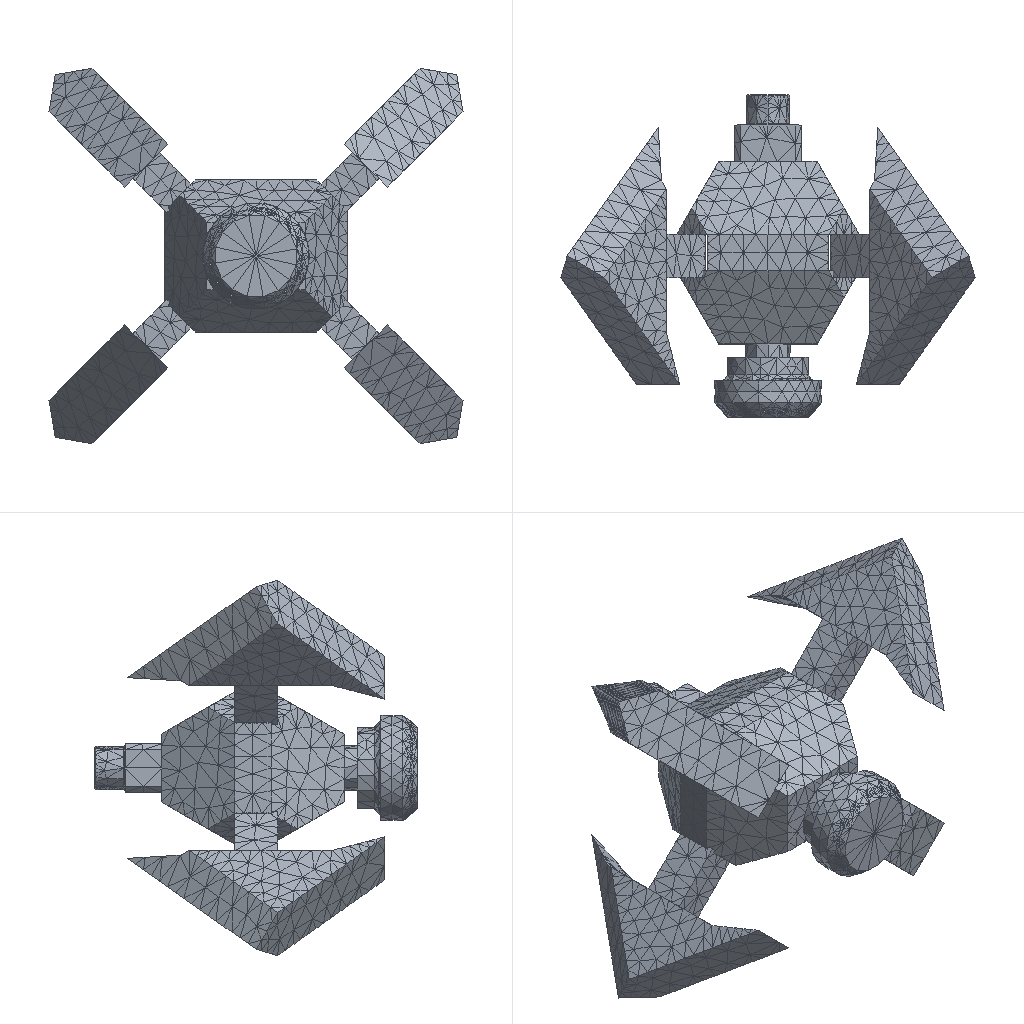Simulation study | ansys workbench
Set-up summary:
category,name,step,type,value,unit,region
solver,ansys_workbench
units,mm-N-s-tonne (MPa),,stated,"/units,MPA"
analysis,LS1,,static
load_step,LS1,LS1,static,nsubst=1; time=1
mesh,nodes,,,44105
mesh,elements,,,24845
element_type,SOLID187,,,22843
element_type,TARGE170,,,815
element_type,CONTA174,,,815
element_type,SURF154,,,230
element_type,SOLID186,,,142
material,Structural Steel,,E,200000,tonne s^-2 mm^-1
material,Structural Steel,,nu,0.3
material,Structural Steel,,density,7.85e-09,tonne mm^-3
material,Structural Steel,,conductivity,60.5,tonne mm s^-3 C^-1
material,Structural Steel,,specific_heat,4.34e+08,mm^2 s^-2 C^-1
material,Structural Steel,,cte,1.2e-05,C^-1
material,Structural Steel,,permeability,10000
material,Structural Steel,,resistivity,0.00017,ohm mm
load,"Define Pressure Using Surface Effect Elements ""__""",LS1,pressure,0.05,,SURF154 #25
load,Define Force Using Surface Effect Elements,LS1,surface-effect pres face 2,-0.01863,,SURF154 #26
bc,Fixed Supports,model,fixed,[dofs=ALL],,_FIXEDSU
contact,Contact Region,,bonded (always),element=CONTA174
contact,Contact Region 2,,bonded (always),element=CONTA174
contact,Contact Region 3,,bonded (always),element=CONTA174
contact,Contact Region 4,,bonded (always),element=CONTA174
contact,Contact Region 5,,bonded (always),element=CONTA174
contact,Contact Region 6,,bonded (always),element=CONTA174
contact,Contact Region 7,,bonded (always),element=CONTA174
contact,Contact Region 8,,bonded (always),element=CONTA174
named_set,_FIXEDSU,,node,980
Ansys APDL input file, long lists of numbers shortened:
/batch
/config,noeldb,1     ! force off writing results to database
*get,_wallstrt,active,,time,wall
! ANSYS input file written by Workbench version 2022 R1
! File used for geometry attach:
/title,wbnew--____ (B5)
! ****** Begin Custom Load Command Snippet ******
/COM, ACT Extensions:
/COM,     LSDYNA, 2021.1
/COM,
! ****** End   Custom Load Command Snippet ******
*DIM,_wb_ProjectScratch_dir,string,248
_wb_ProjectScratch_dir(1) = ''
*DIM,_wb_SolverFiles_dir,string,248
_wb_SolverFiles_dir(1) = ''
*DIM,_wb_userfiles_dir,string,248
_wb_userfiles_dir(1) = ''
/com,--- Data in consistent NMM units. See Solving Units in the help system for more information.
/units,MPA
/nopr
/wb,file,start              !  signify a WB generated input file
/prep7
! Turn off shape checking because checks already performed inside WB mesher.
! See help system for more information.
SHPP,OFF,,NOWARN
/nolist
etcon,set             ! allow ANSYS to choose best KEYOP's for 180x elements, resets any applicable keyopt to MAPDL defaults
/com,*********** Nodes for the whole assembly ***********
nblock,3,,48515
(1i9,3e20.9e3)
        1     5.028046008E+01     2.042995881E+02    -1.157319943E+01
! (44104 more lines like these left out)
-1
/wb,elem,start            !  set before creation of elements
/com,*********** Elements for Body 1 "__|__1" ***********
et,1,187
eblock,19,solid,,1525
(19i9)
        1        1        1        1        0        0        0        0       10        0      143     1288     1380     1470     1477     2782     3319     2784     2785
! (3049 more lines like these left out)
-1
/com,*********** Elements for Body 2 "___|___1" ***********
et,2,187
eblock,19,solid,,9956
(19i9)
        2        2        2        2        0        0        0        0       10        0    13030    29622    30030    29741    29839    43103    43625    43098    43100
! (19911 more lines like these left out)
-1
/com,*********** Elements for Body 3 "____|__-__1" ***********
et,3,186
keyo,3,2,1          ! set full integration on SOLID186
eblock,19,solid,,142
(19i9)
        3        3        3        3        0        0        0        0       20        0        1        7      316       13      153       26      315       20      163
! (283 more lines like these left out)
-1
/com,*********** Elements for Body 4 "___|__2" ***********
et,4,187
eblock,19,solid,,3028
(19i9)
        4        4        4        4        0        0        0        0       10        0     6243    13936    13937    14647    14646    17128    17151    17141    17140
! (6055 more lines like these left out)
-1
/com,*********** Elements for Body 5 "__|__1" ***********
et,5,187
eblock,19,solid,,3759
(19i9)
        5        5        5        5        0        0        0        0       10        0     9271    20224    21134    20732    21129    24359    26317    24356    24358
! (7517 more lines like these left out)
-1
/com,*********** Elements for Body 6 "__|__1[2]" ***********
et,6,187
eblock,19,solid,,1525
(19i9)
        6        6        6        6        0        0        0        0       10        0     4718    10588    10680    10770    10777    12082    12619    12084    12085
! (3049 more lines like these left out)
-1
/com,*********** Elements for Body 7 "__|__1[3]" ***********
et,7,187
eblock,19,solid,,1525
(19i9)
        7        7        7        7        0        0        0        0       10        0     1668     4388     4480     4570     4577     5882     6419     5884     5885
! (3049 more lines like these left out)
-1
/com,*********** Elements for Body 8 "__|__1[4]" ***********
et,8,187
eblock,19,solid,,1525
(19i9)
        8        8        8        8        0        0        0        0       10        0     3193     7488     7580     7670     7677     8982     9519     8984     8985
! (3049 more lines like these left out)
-1
/wb,elem,end               !  done creating elements
/com,*********** Send User Defined Coordinate System(s) ***********
csys,0
toffst,273.15,  ! Temperature offset from absolute zero
/com,*********** Set Reference Temperature ***********
tref,22.
/wb,mat,start              !  starting to send materials
/com,*********** Send Materials ***********
Temperature = 'TEMP' ! Temperature
MP,DENS,1,7.85e-09,	! tonne mm^-3
MP,ALPX,1,1.2e-05,	! C^-1
MP,C,1,434000000,	! mm^2 s^-2 C^-1
MP,KXX,1,60.5,	! tonne mm s^-3 C^-1
MP,RSVX,1,0.00017,	! ohm mm
MP,EX,1,200000,	! tonne s^-2 mm^-1
MP,NUXY,1,0.3,
MP,MURX,1,10000,
Temperature = 'TEMP' ! Temperature
MP,DENS,2,7.85e-09,	! tonne mm^-3
MP,ALPX,2,1.2e-05,	! C^-1
MP,C,2,434000000,	! mm^2 s^-2 C^-1
MP,KXX,2,60.5,	! tonne mm s^-3 C^-1
MP,RSVX,2,0.00017,	! ohm mm
MP,EX,2,200000,	! tonne s^-2 mm^-1
MP,NUXY,2,0.3,
MP,MURX,2,10000,
Temperature = 'TEMP' ! Temperature
MP,DENS,3,7.85e-09,	! tonne mm^-3
MP,ALPX,3,1.2e-05,	! C^-1
MP,C,3,434000000,	! mm^2 s^-2 C^-1
MP,KXX,3,60.5,	! tonne mm s^-3 C^-1
MP,RSVX,3,0.00017,	! ohm mm
MP,EX,3,200000,	! tonne s^-2 mm^-1
MP,NUXY,3,0.3,
MP,MURX,3,10000,
Temperature = 'TEMP' ! Temperature
MP,DENS,4,7.85e-09,	! tonne mm^-3
MP,ALPX,4,1.2e-05,	! C^-1
MP,C,4,434000000,	! mm^2 s^-2 C^-1
MP,KXX,4,60.5,	! tonne mm s^-3 C^-1
MP,RSVX,4,0.00017,	! ohm mm
MP,EX,4,200000,	! tonne s^-2 mm^-1
MP,NUXY,4,0.3,
MP,MURX,4,10000,
Temperature = 'TEMP' ! Temperature
MP,DENS,5,7.85e-09,	! tonne mm^-3
MP,ALPX,5,1.2e-05,	! C^-1
MP,C,5,434000000,	! mm^2 s^-2 C^-1
MP,KXX,5,60.5,	! tonne mm s^-3 C^-1
MP,RSVX,5,0.00017,	! ohm mm
MP,EX,5,200000,	! tonne s^-2 mm^-1
MP,NUXY,5,0.3,
MP,MURX,5,10000,
Temperature = 'TEMP' ! Temperature
MP,DENS,6,7.85e-09,	! tonne mm^-3
MP,ALPX,6,1.2e-05,	! C^-1
MP,C,6,434000000,	! mm^2 s^-2 C^-1
MP,KXX,6,60.5,	! tonne mm s^-3 C^-1
MP,RSVX,6,0.00017,	! ohm mm
MP,EX,6,200000,	! tonne s^-2 mm^-1
MP,NUXY,6,0.3,
MP,MURX,6,10000,
Temperature = 'TEMP' ! Temperature
MP,DENS,7,7.85e-09,	! tonne mm^-3
MP,ALPX,7,1.2e-05,	! C^-1
MP,C,7,434000000,	! mm^2 s^-2 C^-1
MP,KXX,7,60.5,	! tonne mm s^-3 C^-1
MP,RSVX,7,0.00017,	! ohm mm
MP,EX,7,200000,	! tonne s^-2 mm^-1
MP,NUXY,7,0.3,
MP,MURX,7,10000,
Temperature = 'TEMP' ! Temperature
MP,DENS,8,7.85e-09,	! tonne mm^-3
MP,ALPX,8,1.2e-05,	! C^-1
MP,C,8,434000000,	! mm^2 s^-2 C^-1
MP,KXX,8,60.5,	! tonne mm s^-3 C^-1
MP,RSVX,8,0.00017,	! ohm mm
MP,EX,8,200000,	! tonne s^-2 mm^-1
MP,NUXY,8,0.3,
MP,MURX,8,10000,
/wb,mat,end                !  done sending materials
!************************* Model Summary ********************
!__|__1,	结构钢,	matid,	1
!___|___1,	结构钢,	matid,	2
!____|__-__1,	结构钢,	matid,	3
!___|__2,	结构钢,	matid,	4
!__|__1,	结构钢,	matid,	5
!__|__1[2],	结构钢,	matid,	6
!__|__1[3],	结构钢,	matid,	7
!__|__1[4],	结构钢,	matid,	8
!************************* End Model Summary ********************
! get the diagonal of the bounding box. Needed later for other things
*get,_xmin,node,,mnloc,x
*get,_ymin,node,,mnloc,y
*get,_zmin,node,,mnloc,z
*get,_xmax,node,,mxloc,x
*get,_ymax,node,,mxloc,y
*get,_zmax,node,,mxloc,z
_ASMDIAG=(_xmax-_xmin)*(_xmax-_xmin)+(_ymax-_ymin)*(_ymax-_ymin)+(_zmax-_zmin)*(_zmax-_zmin)
_ASMDIAG=SQRT(_ASMDIAG)
/wb,contact,start          !  starting to send contact
/com,*********** Create Contact "接触区域" ***********
/com,            Real Constant Set For Above Contact Is 10 & 9
*set,tid,10
*set,cid,9
r,tid
r,cid
et,tid,170
et,cid,174
eblock,10,,,15
(15i9)
    35494       10       10       10        0     1151     1329     1666     1666     1742     3103     1666     1745
! (14 more lines like these left out)
-1
eblock,10,,,15
(15i9)
    35509        9        9        9        0     1151     1329     1666     1666     1742     3103     1666     1745
! (14 more lines like these left out)
-1
eblock,10,,,28
(15i9)
    35524        9       10        9        0    19932    20349    20363    20363    22243    24933    20363    22245
! (27 more lines like these left out)
-1
eblock,10,,,28
(15i9)
    35552       10        9       10        0    19932    20349    20363    20363    22243    24933    20363    22245
! (27 more lines like these left out)
-1
keyo,cid,8,2               ! auto create asymmetric contact (from Program Controlled setting)
keyo,cid,10,0              ! adjust contact stiffness each NR iteration (from Program Controlled setting)
keyo,cid,12,5              ! bonded always
keyo,cid,18,1              ! small sliding turned on by application
keyo,cid,2,0               ! augmented Lagrange (from Program Controlled setting)
keyo,cid,4,0               ! on Gauss point (from Program Controlled setting)
keyo,cid,9,1               ! ignore initial gaps/penetration
keyo,cid,7,0               ! No Prediction
rmod,tid,3,10.      ! FKN
rmod,tid,5,0.       ! ICONT
rmod,tid,6,0.       ! PINB
rmod,tid,10,0.      ! CNOF
rmod,tid,12,0.      ! FKT
rmod,tid,36,47      ! WB DSID
rmod,cid,3,10.      ! FKN
rmod,cid,5,0.       ! ICONT
rmod,cid,6,0.       ! PINB
rmod,cid,10,0.      ! CNOF
rmod,cid,12,0.      ! FKT
rmod,cid,36,47      ! WB DSID
/com,*********** Create Contact "接触区域 2" ***********
/com,            Real Constant Set For Above Contact Is 12 & 11
*set,tid,12
*set,cid,11
r,tid
r,cid
et,tid,170
et,cid,174
eblock,10,,,31
(15i9)
    35580       12       12       12        0    28004    28003    28008    28008    33221    33222    28008    33234
! (30 more lines like these left out)
-1
eblock,10,,,31
(15i9)
    35611       11       11       11        0    28004    28003    28008    28008    33221    33222    28008    33234
! (30 more lines like these left out)
-1
eblock,10,,,22
(15i9)
    35642       11       12       11        0    13548    13549    13928    13928    14687    14696    13928    14691
! (21 more lines like these left out)
-1
eblock,10,,,22
(15i9)
    35664       12       11       12        0    13548    13549    13928    13928    14687    14696    13928    14691
! (21 more lines like these left out)
-1
keyo,cid,8,2               ! auto create asymmetric contact (from Program Controlled setting)
keyo,cid,10,0              ! adjust contact stiffness each NR iteration (from Program Controlled setting)
keyo,cid,12,5              ! bonded always
keyo,cid,18,1              ! small sliding turned on by application
keyo,cid,2,0               ! augmented Lagrange (from Program Controlled setting)
keyo,cid,4,0               ! on Gauss point (from Program Controlled setting)
keyo,cid,9,1               ! ignore initial gaps/penetration
keyo,cid,7,0               ! No Prediction
rmod,tid,3,10.      ! FKN
rmod,tid,5,0.       ! ICONT
rmod,tid,6,0.       ! PINB
rmod,tid,10,0.      ! CNOF
rmod,tid,12,0.      ! FKT
rmod,tid,36,50      ! WB DSID
rmod,cid,3,10.      ! FKN
rmod,cid,5,0.       ! ICONT
rmod,cid,6,0.       ! PINB
rmod,cid,10,0.      ! CNOF
rmod,cid,12,0.      ! FKT
rmod,cid,36,50      ! WB DSID
/com,*********** Create Contact "接触区域 3" ***********
/com,            Real Constant Set For Above Contact Is 14 & 13
*set,tid,14
*set,cid,13
r,tid
r,cid
et,tid,170
et,cid,174
eblock,10,,,302
(15i9)
    35686       14       14       14        0    28259    30047    29172    29172    35197    40184    29172    35194
! (301 more lines like these left out)
-1
eblock,10,,,302
(15i9)
    35988       13       13       13        0    28259    30047    29172    29172    35197    40184    29172    35194
! (301 more lines like these left out)
-1
eblock,10,,,32
(15i9)
    36290       13       14       13        0    20286    19840    19845    19845    21521    21519    19845    21554
! (31 more lines like these left out)
-1
eblock,10,,,32
(15i9)
    36322       14       13       14        0    20286    19840    19845    19845    21521    21519    19845    21554
! (31 more lines like these left out)
-1
keyo,cid,8,2               ! auto create asymmetric contact (from Program Controlled setting)
keyo,cid,10,0              ! adjust contact stiffness each NR iteration (from Program Controlled setting)
keyo,cid,12,5              ! bonded always
keyo,cid,18,1              ! small sliding turned on by application
keyo,cid,2,0               ! augmented Lagrange (from Program Controlled setting)
keyo,cid,4,0               ! on Gauss point (from Program Controlled setting)
keyo,cid,9,1               ! ignore initial gaps/penetration
keyo,cid,7,0               ! No Prediction
rmod,tid,3,10.      ! FKN
rmod,tid,5,0.       ! ICONT
rmod,tid,6,0.       ! PINB
rmod,tid,10,0.      ! CNOF
rmod,tid,12,0.      ! FKT
rmod,tid,36,53      ! WB DSID
rmod,cid,3,10.      ! FKN
rmod,cid,5,0.       ! ICONT
rmod,cid,6,0.       ! PINB
rmod,cid,10,0.      ! CNOF
rmod,cid,12,0.      ! FKT
rmod,cid,36,53      ! WB DSID
/com,*********** Create Contact "接触区域 4" ***********
/com,            Real Constant Set For Above Contact Is 16 & 15
*set,tid,16
*set,cid,15
r,tid
r,cid
et,tid,170
et,cid,174
eblock,10,,,40
(15i9)
    36354       16       16       16        0      169      149      167      168      760      759      805      807
! (39 more lines like these left out)
-1
eblock,10,,,40
(15i9)
    36394       15       15       15        0      169      149      167      168      760      759      805      807
! (39 more lines like these left out)
-1
eblock,10,,,23
(15i9)
    36434       15       16       15        0    19863    19862    20716    20716    21692    21694    20716    21698
! (22 more lines like these left out)
-1
eblock,10,,,23
(15i9)
    36457       16       15       16        0    19863    19862    20716    20716    21692    21694    20716    21698
! (22 more lines like these left out)
-1
keyo,cid,8,2               ! auto create asymmetric contact (from Program Controlled setting)
keyo,cid,10,0              ! adjust contact stiffness each NR iteration (from Program Controlled setting)
keyo,cid,12,5              ! bonded always
keyo,cid,18,1              ! small sliding turned on by application
keyo,cid,2,0               ! augmented Lagrange (from Program Controlled setting)
keyo,cid,4,0               ! on Gauss point (from Program Controlled setting)
keyo,cid,9,1               ! ignore initial gaps/penetration
keyo,cid,7,0               ! No Prediction
rmod,tid,3,10.      ! FKN
rmod,tid,5,0.       ! ICONT
rmod,tid,6,0.       ! PINB
rmod,tid,10,0.      ! CNOF
rmod,tid,12,0.      ! FKT
rmod,tid,36,56      ! WB DSID
rmod,cid,3,10.      ! FKN
rmod,cid,5,0.       ! ICONT
rmod,cid,6,0.       ! PINB
rmod,cid,10,0.      ! CNOF
rmod,cid,12,0.      ! FKT
rmod,cid,36,56      ! WB DSID
/com,*********** Create Contact "接触区域 5" ***********
/com,            Real Constant Set For Above Contact Is 18 & 17
*set,tid,18
*set,cid,17
r,tid
r,cid
et,tid,170
et,cid,174
eblock,10,,,127
(15i9)
    36480       18       18       18        0    13548    13549    13928    13928    14687    14696    13928    14691
! (126 more lines like these left out)
-1
eblock,10,,,127
(15i9)
    36607       17       17       17        0    13548    13549    13928    13928    14687    14696    13928    14691
! (126 more lines like these left out)
-1
eblock,10,,,66
(15i9)
    36734       17       18       17        0    19833    20280    20740    20740    21435    24602    20740    21437
! (65 more lines like these left out)
-1
eblock,10,,,66
(15i9)
    36800       18       17       18        0    19833    20280    20740    20740    21435    24602    20740    21437
! (65 more lines like these left out)
-1
keyo,cid,8,2               ! auto create asymmetric contact (from Program Controlled setting)
keyo,cid,10,0              ! adjust contact stiffness each NR iteration (from Program Controlled setting)
keyo,cid,12,5              ! bonded always
keyo,cid,18,1              ! small sliding turned on by application
keyo,cid,2,0               ! augmented Lagrange (from Program Controlled setting)
keyo,cid,4,0               ! on Gauss point (from Program Controlled setting)
keyo,cid,9,1               ! ignore initial gaps/penetration
keyo,cid,7,0               ! No Prediction
rmod,tid,3,10.      ! FKN
rmod,tid,5,0.       ! ICONT
rmod,tid,6,0.       ! PINB
rmod,tid,10,0.      ! CNOF
rmod,tid,12,0.      ! FKT
rmod,tid,36,59      ! WB DSID
rmod,cid,3,10.      ! FKN
rmod,cid,5,0.       ! ICONT
rmod,cid,6,0.       ! PINB
rmod,cid,10,0.      ! CNOF
rmod,cid,12,0.      ! FKT
rmod,cid,36,59      ! WB DSID
/com,*********** Create Contact "接触区域 6" ***********
/com,            Real Constant Set For Above Contact Is 20 & 19
*set,tid,20
*set,cid,19
r,tid
r,cid
et,tid,170
et,cid,174
eblock,10,,,28
(15i9)
    36866       20       20       20        0    19874    20303    20299    20299    21787    24684    20299    21786
! (27 more lines like these left out)
-1
eblock,10,,,28
(15i9)
    36894       19       19       19        0    19874    20303    20299    20299    21787    24684    20299    21786
! (27 more lines like these left out)
-1
eblock,10,,,15
(15i9)
    36922       19       20       19        0    10451    10629    10966    10966    11042    12403    10966    11045
! (14 more lines like these left out)
-1
eblock,10,,,15
(15i9)
    36937       20       19       20        0    10451    10629    10966    10966    11042    12403    10966    11045
! (14 more lines like these left out)
-1
keyo,cid,8,2               ! auto create asymmetric contact (from Program Controlled setting)
keyo,cid,10,0              ! adjust contact stiffness each NR iteration (from Program Controlled setting)
keyo,cid,12,5              ! bonded always
keyo,cid,18,1              ! small sliding turned on by application
keyo,cid,2,0               ! augmented Lagrange (from Program Controlled setting)
keyo,cid,4,0               ! on Gauss point (from Program Controlled setting)
keyo,cid,9,1               ! ignore initial gaps/penetration
keyo,cid,7,0               ! No Prediction
rmod,tid,3,10.      ! FKN
rmod,tid,5,0.       ! ICONT
rmod,tid,6,0.       ! PINB
rmod,tid,10,0.      ! CNOF
rmod,tid,12,0.      ! FKT
rmod,tid,36,62      ! WB DSID
rmod,cid,3,10.      ! FKN
rmod,cid,5,0.       ! ICONT
rmod,cid,6,0.       ! PINB
rmod,cid,10,0.      ! CNOF
rmod,cid,12,0.      ! FKT
rmod,cid,36,62      ! WB DSID
/com,*********** Create Contact "接触区域 7" ***********
/com,            Real Constant Set For Above Contact Is 22 & 21
*set,tid,22
*set,cid,21
r,tid
r,cid
et,tid,170
et,cid,174
eblock,10,,,28
(15i9)
    36952       22       22       22        0    19990    20668    19991    19991    22657    22663    19991    22655
! (27 more lines like these left out)
-1
eblock,10,,,28
(15i9)
    36980       21       21       21        0    19990    20668    19991    19991    22657    22663    19991    22655
! (27 more lines like these left out)
-1
eblock,10,,,15
(15i9)
    37008       21       22       21        0     4251     4429     4766     4766     4842     6203     4766     4845
! (14 more lines like these left out)
-1
eblock,10,,,15
(15i9)
    37023       22       21       22        0     4251     4429     4766     4766     4842     6203     4766     4845
! (14 more lines like these left out)
-1
keyo,cid,8,2               ! auto create asymmetric contact (from Program Controlled setting)
keyo,cid,10,0              ! adjust contact stiffness each NR iteration (from Program Controlled setting)
keyo,cid,12,5              ! bonded always
keyo,cid,18,1              ! small sliding turned on by application
keyo,cid,2,0               ! augmented Lagrange (from Program Controlled setting)
keyo,cid,4,0               ! on Gauss point (from Program Controlled setting)
keyo,cid,9,1               ! ignore initial gaps/penetration
keyo,cid,7,0               ! No Prediction
rmod,tid,3,10.      ! FKN
rmod,tid,5,0.       ! ICONT
rmod,tid,6,0.       ! PINB
rmod,tid,10,0.      ! CNOF
rmod,tid,12,0.      ! FKT
rmod,tid,36,65      ! WB DSID
rmod,cid,3,10.      ! FKN
rmod,cid,5,0.       ! ICONT
rmod,cid,6,0.       ! PINB
rmod,cid,10,0.      ! CNOF
rmod,cid,12,0.      ! FKT
rmod,cid,36,65      ! WB DSID
/com,*********** Create Contact "接触区域 8" ***********
/com,            Real Constant Set For Above Contact Is 24 & 23
*set,tid,24
*set,cid,23
r,tid
r,cid
et,tid,170
et,cid,174
eblock,10,,,28
(15i9)
    37038       24       24       24        0    19984    20673    19985    19985    22623    22627    19985    22619
! (27 more lines like these left out)
-1
eblock,10,,,28
(15i9)
    37066       23       23       23        0    19984    20673    19985    19985    22623    22627    19985    22619
! (27 more lines like these left out)
-1
eblock,10,,,15
(15i9)
    37094       23       24       23        0     7353     7863     7530     7530     7958     9307     7530     7952
! (14 more lines like these left out)
-1
eblock,10,,,15
(15i9)
    37109       24       23       24        0     7353     7863     7530     7530     7958     9307     7530     7952
! (14 more lines like these left out)
-1
keyo,cid,8,2               ! auto create asymmetric contact (from Program Controlled setting)
keyo,cid,10,0              ! adjust contact stiffness each NR iteration (from Program Controlled setting)
keyo,cid,12,5              ! bonded always
keyo,cid,18,1              ! small sliding turned on by application
keyo,cid,2,0               ! augmented Lagrange (from Program Controlled setting)
keyo,cid,4,0               ! on Gauss point (from Program Controlled setting)
keyo,cid,9,1               ! ignore initial gaps/penetration
keyo,cid,7,0               ! No Prediction
rmod,tid,3,10.      ! FKN
rmod,tid,5,0.       ! ICONT
rmod,tid,6,0.       ! PINB
rmod,tid,10,0.      ! CNOF
rmod,tid,12,0.      ! FKT
rmod,tid,36,68      ! WB DSID
rmod,cid,3,10.      ! FKN
rmod,cid,5,0.       ! ICONT
rmod,cid,6,0.       ! PINB
rmod,cid,10,0.      ! CNOF
rmod,cid,12,0.      ! FKT
rmod,cid,36,68      ! WB DSID
nsel,all
esel,all
/wb,contact,end            !  done creating contacts
/golist
/wb,load,start             !  starting to send loads
/com,*********** Fixed Supports ***********
CMBLOCK,_FIXEDSU,NODE,      980
(8i10)
      1201      1204      1205      1206      1209      1210      1211      1212
! (122 more lines like these left out)
cmsel,s,_FIXEDSU
d,all,all
nsel,all
/com,*********** Define Pressure Using Surface Effect Elements "__" ***********
et,25,154
eblock,10,,,134
(15i9)
    37124       25       25       25        0    28037    28040    28041    28041    33494    33529    28041    33495
! (133 more lines like these left out)
-1
esel,s,type,,25
keyop,25,7,0                ! Use deformed area for application of load
esel,all
/com,*********** Define Force Using Surface Effect Elements ***********
local,12,0,0.,0.,0.,0.,0.,0.
csys,0
et,26,154
eblock,10,,,96
(15i9)
    37258       26       26       26       12     1151     1329     1666     1666     1742     3103     1666     1745
! (95 more lines like these left out)
-1
esel,s,type,,26
keyop,26,2,1                ! Apply load in local coordinate system
keyop,26,7,1                ! Use original area so load is constant in large deformation
esel,all
esel,all
/gst,on,on
fini
*get,_numnode,node,0,count
*get,_numelem,elem,0,count
*get, _MAXELEMNUM, elem, 0, NUM, MAX
*get, _MAXNODENUM, node, 0, NUM, MAX
*get, _MAXELEMTYPE, etyp, 0, NUM, MAX
*get, _MAXREALCONST, real, 0, NUM, MAX
/go
/wb,load,end               !  done creating loads
/com,--- Number of total nodes = %_numnode%
/com,--- Number of contact elements = 1860
/com,--- Number of spring elements = 0
/com,--- Number of bearing elements = 0
/com,--- Number of solid elements = 22985
/com,--- Number of condensed parts = 0
/com,--- Number of total elements = %_numelem%
*get,_wallbsol,active,,time,wall
/com,****************************************************************************
/com,*************************    SOLUTION       ********************************
/com,****************************************************************************
/solu
antype,0                   ! static analysis
_thickRatio=0.125   ! Ratio of thick parts in the model
eqsl,sparse,,,,,1
cntr,print,1               ! print out contact info and also make no initial contact an error
dmpoption,emat,no             ! Don't combine emat file for DANSYS
dmpoption,esav,no             ! Don't combine esav file for DANSYS
nldiag,cont,iter           ! print out contact info each equilibrium iteration
rescontrol,,none                 ! Do not keep any restart files
/com,****************************************************
/com,******************* SOLVE FOR LS 1 OF 1 ****************
esel,s,type,,25
nsle
sf,all,pres,5.e-002
nsel,all
esel,all
esel,s,type,,26
nsle
sfe,all,1,pres,1,0.
sfe,all,2,pres,1,-1.86289120715294e-002
sfe,all,3,pres,1,0.
nsel,all
esel,all
esel,all
/nopr
/gopr
nsub,1,1,1
time,1.
outres,erase
outres,all,none
outres,nsol,all,
outres,rsol,all
outres,eangl,all
outres,etmp,all
outres,veng,all
outres,strs,all,
outres,epel,all,
outres,eppl,all,
outres,cont,all,
! *********** WB SOLVE COMMAND ***********
! check interactive state
*get,ANSINTER_,active,,int
*if,ANSINTER_,ne,0,then
/eof
*endif
solve
/com *************** Write FE CONNECTORS *********
CEWRITE,file,ce,,INTE
/com,****************************************************
/com,*************** FINISHED SOLVE FOR LS 1 *************
*get,_wallasol,active,,time,wall
/nopr
*get,_numnode,node,0,count
*get,_numelem,elem,0,count
*get, _MAXELEMNUM, elem, 0, NUM, MAX
*get, _MAXNODENUM, node, 0, NUM, MAX,,,INTERNAL
*get, _MAXELEMTYPE, etyp, 0, NUM, MAX
*get, _MAXREALCONST, real, 0, NUM, MAX
/gopr
/post1
xmlo,ENCODING,ISO-8859-1
xmlo,parm
/xml,parm,xml
fini
/gopr
*get,_walldone,active,,time,wall
_preptime=(_wallbsol-_wallstrt)*3600
_solvtime=(_wallasol-_wallbsol)*3600
_posttime=(_walldone-_wallasol)*3600
_totaltim=(_walldone-_wallstrt)*3600
*get,_dlbratio,active,0,solu,dlbr
*get,_combtime,active,0,solu,comb
*get,_ssmode,active,0,solu,ssmm
*get,_ndofs,active,0,solu,ndof
*get,_sol_end_time,active,0,set,time
*if,_sol_end_time,eq,1.,then
/fclean				!clean distributed files
*endif
/com,--- Total number of nodes = %_numnode%
/com,--- Total number of elements = %_numelem%
/com,--- Element load balance ratio = %_dlbratio%
/com,--- Time to combine distributed files = %_combtime%
/com,--- Sparse memory mode = %_ssmode%
/com,--- Number of DOF = %_ndofs%
/wb,file,end               ! done with WB generated input
Results summary:
result,analyses[0].index,,,1
result,analyses[0].system,,,SYS-1
result,analyses[0].deck,,,deck.dat
result,analyses[0].solve_status,,,completed
result,analyses[0].analysis_type,,,static
result,analyses[0].physics,,,mechanical
result,analyses[0].unit_system,,,"NMM: mm, ton, N, s, mV, mA, degC"
result,analyses[0].n_sets,,,1
result,analyses[0].load_steps[0].set,set=1,,1
result,analyses[0].load_steps[0].time_or_freq,set=1,,1
result,analyses[0].load_steps[0].max_displacement_magnitude,set=1,,0.0005239
result,analyses[0].load_steps[0].max_von_mises_nodal,set=1,,0.4527
result,analyses[0].load_steps[0].reaction_force_sum_xyz[1],set=1,,-0.0003939
result,analyses[0].load_steps[0].reaction_force_sum_xyz[2],set=1,,622.067
result,analyses[0].load_steps[0].reaction_force_sum_xyz[3],set=1,,0.0005402